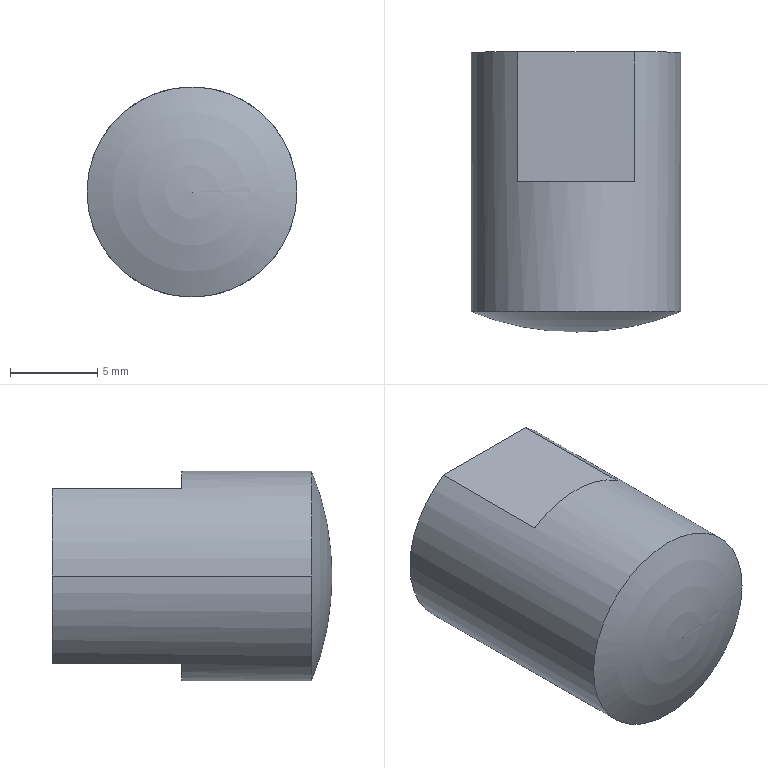Part | NX | 1 solid | 12 faces | box 12 x 16 x 12 mm | volume 1561 mm3 | plane 5 | cylinder 4 | cone 2 | sphere 1 | commonest cylinder face diameters 4.2 x2 12 x2
STEP:
#1=CARTESIAN_POINT('',(6.,-2.832,0.));
#2=VERTEX_POINT('',#1);
#3=CARTESIAN_POINT('',(-6.,-2.832,0.));
#4=VERTEX_POINT('',#3);
#5=CARTESIAN_POINT('',(0.,-2.832,0.));
#6=DIRECTION('',(0.,1.,0.));
#7=DIRECTION('',(1.,0.,0.));
#8=AXIS2_PLACEMENT_3D('',#5,#6,#7);
#9=CIRCLE('',#8,6.);
#10=EDGE_CURVE('',#2,#4,#9,.T.);
#11=ORIENTED_EDGE('',*,*,#10,.F.);
#12=CARTESIAN_POINT('',(0.,-2.832,0.));
#13=DIRECTION('',(0.,1.,0.));
#14=DIRECTION('',(1.,0.,0.));
#15=AXIS2_PLACEMENT_3D('',#12,#13,#14);
#16=CIRCLE('',#15,6.);
#17=EDGE_CURVE('',#4,#2,#16,.T.);
#18=ORIENTED_EDGE('',*,*,#17,.F.);
#19=EDGE_LOOP('',(#11,#18));
#20=FACE_BOUND('',#19,.T.);
#21=CARTESIAN_POINT('',(0.,12.,0.));
#22=DIRECTION('',(0.,1.,0.));
#23=DIRECTION('',(1.,0.,0.));
#24=AXIS2_PLACEMENT_3D('',#21,#22,#23);
#25=SPHERICAL_SURFACE('',#24,16.);
#26=ADVANCED_FACE('',(#20),#25,.T.);
#27=CARTESIAN_POINT('',(-2.1,4.,0.));
#28=VERTEX_POINT('',#27);
#29=CARTESIAN_POINT('',(2.1,4.,0.));
#30=VERTEX_POINT('',#29);
#31=CARTESIAN_POINT('',(0.,4.,0.));
#32=DIRECTION('',(0.,-1.,0.));
#33=DIRECTION('',(1.,0.,0.));
#34=AXIS2_PLACEMENT_3D('',#31,#32,#33);
#35=CIRCLE('',#34,2.1);
#36=EDGE_CURVE('',#28,#30,#35,.T.);
#37=ORIENTED_EDGE('',*,*,#36,.T.);
#38=CARTESIAN_POINT('',(2.1,12.,0.));
#39=VERTEX_POINT('',#38);
#40=CARTESIAN_POINT('',(2.1,2.275,0.));
#41=DIRECTION('',(0.,1.,0.));
#42=VECTOR('',#41,1000.);
#43=LINE('',#40,#42);
#44=EDGE_CURVE('',#30,#39,#43,.T.);
#45=ORIENTED_EDGE('',*,*,#44,.T.);
#46=CARTESIAN_POINT('',(-2.1,12.,0.));
#47=VERTEX_POINT('',#46);
#48=CARTESIAN_POINT('',(0.,12.,0.));
#49=DIRECTION('',(0.,1.,0.));
#50=DIRECTION('',(-1.,0.,0.));
#51=AXIS2_PLACEMENT_3D('',#48,#49,#50);
#52=CIRCLE('',#51,2.1);
#53=EDGE_CURVE('',#39,#47,#52,.T.);
#54=ORIENTED_EDGE('',*,*,#53,.T.);
#55=CARTESIAN_POINT('',(-2.1,2.275,0.));
#56=DIRECTION('',(0.,1.,0.));
#57=VECTOR('',#56,1000.);
#58=LINE('',#55,#57);
#59=EDGE_CURVE('',#28,#47,#58,.T.);
#60=ORIENTED_EDGE('',*,*,#59,.F.);
#61=EDGE_LOOP('',(#37,#45,#54,#60));
#62=FACE_BOUND('',#61,.T.);
#63=CARTESIAN_POINT('',(0.,2.275,0.));
#64=DIRECTION('',(0.,1.,0.));
#65=DIRECTION('',(1.,0.,0.));
#66=AXIS2_PLACEMENT_3D('',#63,#64,#65);
#67=CYLINDRICAL_SURFACE('',#66,2.1);
#68=ADVANCED_FACE('',(#62),#67,.F.);
#69=ORIENTED_EDGE('',*,*,#10,.T.);
#70=CARTESIAN_POINT('',(-6.,12.,0.));
#71=VERTEX_POINT('',#70);
#72=CARTESIAN_POINT('',(-6.,12.8,0.));
#73=DIRECTION('',(0.,-1.,0.));
#74=VECTOR('',#73,1000.);
#75=LINE('',#72,#74);
#76=EDGE_CURVE('',#71,#4,#75,.T.);
#77=ORIENTED_EDGE('',*,*,#76,.F.);
#78=CARTESIAN_POINT('',(-3.317,12.,-5.));
#79=VERTEX_POINT('',#78);
#80=CARTESIAN_POINT('',(0.,12.,0.));
#81=DIRECTION('',(0.,-1.,0.));
#82=DIRECTION('',(-1.,0.,0.));
#83=AXIS2_PLACEMENT_3D('',#80,#81,#82);
#84=CIRCLE('',#83,6.);
#85=EDGE_CURVE('',#71,#79,#84,.T.);
#86=ORIENTED_EDGE('',*,*,#85,.T.);
#87=CARTESIAN_POINT('',(-3.317,4.584,-5.));
#88=VERTEX_POINT('',#87);
#89=CARTESIAN_POINT('',(-3.317,4.584,-5.));
#90=DIRECTION('',(0.,1.,0.));
#91=VECTOR('',#90,1000.);
#92=LINE('',#89,#91);
#93=EDGE_CURVE('',#88,#79,#92,.T.);
#94=ORIENTED_EDGE('',*,*,#93,.F.);
#95=CARTESIAN_POINT('',(3.317,4.584,-5.));
#96=VERTEX_POINT('',#95);
#97=CARTESIAN_POINT('',(0.,4.584,0.));
#98=DIRECTION('',(0.,-1.,0.));
#99=DIRECTION('',(-0.5528,0.,-0.8333));
#100=AXIS2_PLACEMENT_3D('',#97,#98,#99);
#101=CIRCLE('',#100,6.);
#102=EDGE_CURVE('',#88,#96,#101,.T.);
#103=ORIENTED_EDGE('',*,*,#102,.T.);
#104=CARTESIAN_POINT('',(3.317,12.,-5.));
#105=VERTEX_POINT('',#104);
#106=CARTESIAN_POINT('',(3.317,12.,-5.));
#107=DIRECTION('',(0.,-1.,0.));
#108=VECTOR('',#107,1000.);
#109=LINE('',#106,#108);
#110=EDGE_CURVE('',#105,#96,#109,.T.);
#111=ORIENTED_EDGE('',*,*,#110,.F.);
#112=CARTESIAN_POINT('',(6.,12.,0.));
#113=VERTEX_POINT('',#112);
#114=CARTESIAN_POINT('',(0.,12.,0.));
#115=DIRECTION('',(0.,-1.,0.));
#116=DIRECTION('',(0.5528,0.,-0.8333));
#117=AXIS2_PLACEMENT_3D('',#114,#115,#116);
#118=CIRCLE('',#117,6.);
#119=EDGE_CURVE('',#105,#113,#118,.T.);
#120=ORIENTED_EDGE('',*,*,#119,.T.);
#121=CARTESIAN_POINT('',(6.,12.8,0.));
#122=DIRECTION('',(0.,-1.,0.));
#123=VECTOR('',#122,1000.);
#124=LINE('',#121,#123);
#125=EDGE_CURVE('',#113,#2,#124,.T.);
#126=ORIENTED_EDGE('',*,*,#125,.T.);
#127=EDGE_LOOP('',(#69,#77,#86,#94,#103,#111,#120,#126));
#128=FACE_BOUND('',#127,.T.);
#129=CARTESIAN_POINT('',(0.,12.8,0.));
#130=DIRECTION('',(0.,-1.,0.));
#131=DIRECTION('',(1.,0.,0.));
#132=AXIS2_PLACEMENT_3D('',#129,#130,#131);
#133=CYLINDRICAL_SURFACE('',#132,6.);
#134=ADVANCED_FACE('',(#128),#133,.T.);
#135=ORIENTED_EDGE('',*,*,#85,.F.);
#136=CARTESIAN_POINT('',(-3.317,12.,5.));
#137=VERTEX_POINT('',#136);
#138=CARTESIAN_POINT('',(0.,12.,0.));
#139=DIRECTION('',(0.,-1.,0.));
#140=DIRECTION('',(-1.,0.,0.));
#141=AXIS2_PLACEMENT_3D('',#138,#139,#140);
#142=CIRCLE('',#141,6.);
#143=EDGE_CURVE('',#137,#71,#142,.T.);
#144=ORIENTED_EDGE('',*,*,#143,.F.);
#145=CARTESIAN_POINT('',(3.317,12.,5.));
#146=VERTEX_POINT('',#145);
#147=CARTESIAN_POINT('',(-3.317,12.,5.));
#148=DIRECTION('',(1.,0.,0.));
#149=VECTOR('',#148,1000.);
#150=LINE('',#147,#149);
#151=EDGE_CURVE('',#137,#146,#150,.T.);
#152=ORIENTED_EDGE('',*,*,#151,.T.);
#153=CARTESIAN_POINT('',(0.,12.,0.));
#154=DIRECTION('',(0.,-1.,0.));
#155=DIRECTION('',(0.5528,0.,-0.8333));
#156=AXIS2_PLACEMENT_3D('',#153,#154,#155);
#157=CIRCLE('',#156,6.);
#158=EDGE_CURVE('',#113,#146,#157,.T.);
#159=ORIENTED_EDGE('',*,*,#158,.F.);
#160=ORIENTED_EDGE('',*,*,#119,.F.);
#161=CARTESIAN_POINT('',(-3.317,12.,-5.));
#162=DIRECTION('',(1.,0.,0.));
#163=VECTOR('',#162,1000.);
#164=LINE('',#161,#163);
#165=EDGE_CURVE('',#79,#105,#164,.T.);
#166=ORIENTED_EDGE('',*,*,#165,.F.);
#167=EDGE_LOOP('',(#135,#144,#152,#159,#160,#166));
#168=FACE_BOUND('',#167,.T.);
#169=ORIENTED_EDGE('',*,*,#53,.F.);
#170=CARTESIAN_POINT('',(0.,12.,0.));
#171=DIRECTION('',(0.,1.,0.));
#172=DIRECTION('',(-1.,0.,0.));
#173=AXIS2_PLACEMENT_3D('',#170,#171,#172);
#174=CIRCLE('',#173,2.1);
#175=EDGE_CURVE('',#47,#39,#174,.T.);
#176=ORIENTED_EDGE('',*,*,#175,.F.);
#177=EDGE_LOOP('',(#169,#176));
#178=FACE_BOUND('',#177,.T.);
#179=CARTESIAN_POINT('',(0.,12.,0.));
#180=DIRECTION('',(0.,-1.,0.));
#181=DIRECTION('',(0.,0.,-1.));
#182=AXIS2_PLACEMENT_3D('',#179,#180,#181);
#183=PLANE('',#182);
#184=ADVANCED_FACE('',(#168,#178),#183,.F.);
#185=CARTESIAN_POINT('',(0.,2.738,0.));
#186=VERTEX_POINT('',#185);
#187=CARTESIAN_POINT('',(-1.071,3.382,0.));
#188=DIRECTION('',(-0.8572,0.515,0.));
#189=VECTOR('',#188,1000.);
#190=LINE('',#187,#189);
#191=EDGE_CURVE('',#28,#186,#190,.F.);
#192=ORIENTED_EDGE('',*,*,#191,.F.);
#193=CARTESIAN_POINT('',(0.,4.,0.));
#194=DIRECTION('',(0.,-1.,0.));
#195=DIRECTION('',(1.,0.,0.));
#196=AXIS2_PLACEMENT_3D('',#193,#194,#195);
#197=CIRCLE('',#196,2.1);
#198=EDGE_CURVE('',#30,#28,#197,.T.);
#199=ORIENTED_EDGE('',*,*,#198,.F.);
#200=CARTESIAN_POINT('',(1.071,3.382,0.));
#201=DIRECTION('',(0.8572,0.515,0.));
#202=VECTOR('',#201,1000.);
#203=LINE('',#200,#202);
#204=EDGE_CURVE('',#30,#186,#203,.F.);
#205=ORIENTED_EDGE('',*,*,#204,.T.);
#206=EDGE_LOOP('',(#192,#199,#205));
#207=FACE_BOUND('',#206,.T.);
#208=CARTESIAN_POINT('',(0.,3.382,0.));
#209=DIRECTION('',(0.,1.,0.));
#210=DIRECTION('',(1.,0.,0.));
#211=AXIS2_PLACEMENT_3D('',#208,#209,#210);
#212=CONICAL_SURFACE('',#211,1.071,1.03);
#213=ADVANCED_FACE('',(#207),#212,.F.);
#214=ORIENTED_EDGE('',*,*,#93,.T.);
#215=ORIENTED_EDGE('',*,*,#165,.T.);
#216=ORIENTED_EDGE('',*,*,#110,.T.);
#217=CARTESIAN_POINT('',(3.317,4.584,-5.));
#218=DIRECTION('',(-1.,0.,0.));
#219=VECTOR('',#218,1000.);
#220=LINE('',#217,#219);
#221=EDGE_CURVE('',#96,#88,#220,.T.);
#222=ORIENTED_EDGE('',*,*,#221,.T.);
#223=EDGE_LOOP('',(#214,#215,#216,#222));
#224=FACE_BOUND('',#223,.T.);
#225=CARTESIAN_POINT('',(-7.2,4.584,-5.));
#226=DIRECTION('',(0.,0.,1.));
#227=DIRECTION('',(1.,0.,0.));
#228=AXIS2_PLACEMENT_3D('',#225,#226,#227);
#229=PLANE('',#228);
#230=ADVANCED_FACE('',(#224),#229,.F.);
#231=ORIENTED_EDGE('',*,*,#102,.F.);
#232=ORIENTED_EDGE('',*,*,#221,.F.);
#233=EDGE_LOOP('',(#231,#232));
#234=FACE_BOUND('',#233,.T.);
#235=CARTESIAN_POINT('',(-7.2,4.584,-6.));
#236=DIRECTION('',(0.,-1.,0.));
#237=DIRECTION('',(0.,0.,-1.));
#238=AXIS2_PLACEMENT_3D('',#235,#236,#237);
#239=PLANE('',#238);
#240=ADVANCED_FACE('',(#234),#239,.F.);
#241=ORIENTED_EDGE('',*,*,#151,.F.);
#242=CARTESIAN_POINT('',(-3.317,4.584,5.));
#243=VERTEX_POINT('',#242);
#244=CARTESIAN_POINT('',(-3.317,12.,5.));
#245=DIRECTION('',(0.,-1.,0.));
#246=VECTOR('',#245,1000.);
#247=LINE('',#244,#246);
#248=EDGE_CURVE('',#137,#243,#247,.T.);
#249=ORIENTED_EDGE('',*,*,#248,.T.);
#250=CARTESIAN_POINT('',(3.317,4.584,5.));
#251=VERTEX_POINT('',#250);
#252=CARTESIAN_POINT('',(3.317,4.584,5.));
#253=DIRECTION('',(-1.,0.,0.));
#254=VECTOR('',#253,1000.);
#255=LINE('',#252,#254);
#256=EDGE_CURVE('',#251,#243,#255,.T.);
#257=ORIENTED_EDGE('',*,*,#256,.F.);
#258=CARTESIAN_POINT('',(3.317,4.584,5.));
#259=DIRECTION('',(0.,1.,0.));
#260=VECTOR('',#259,1000.);
#261=LINE('',#258,#260);
#262=EDGE_CURVE('',#251,#146,#261,.T.);
#263=ORIENTED_EDGE('',*,*,#262,.T.);
#264=EDGE_LOOP('',(#241,#249,#257,#263));
#265=FACE_BOUND('',#264,.T.);
#266=CARTESIAN_POINT('',(-7.2,12.,5.));
#267=DIRECTION('',(0.,0.,-1.));
#268=DIRECTION('',(0.,-1.,0.));
#269=AXIS2_PLACEMENT_3D('',#266,#267,#268);
#270=PLANE('',#269);
#271=ADVANCED_FACE('',(#265),#270,.F.);
#272=CARTESIAN_POINT('',(0.,4.584,0.));
#273=DIRECTION('',(0.,-1.,0.));
#274=DIRECTION('',(0.5528,0.,0.8333));
#275=AXIS2_PLACEMENT_3D('',#272,#273,#274);
#276=CIRCLE('',#275,6.);
#277=EDGE_CURVE('',#251,#243,#276,.T.);
#278=ORIENTED_EDGE('',*,*,#277,.F.);
#279=ORIENTED_EDGE('',*,*,#256,.T.);
#280=EDGE_LOOP('',(#278,#279));
#281=FACE_BOUND('',#280,.T.);
#282=CARTESIAN_POINT('',(-7.2,4.584,5.));
#283=DIRECTION('',(0.,-1.,0.));
#284=DIRECTION('',(0.,0.,-1.));
#285=AXIS2_PLACEMENT_3D('',#282,#283,#284);
#286=PLANE('',#285);
#287=ADVANCED_FACE('',(#281),#286,.F.);
#288=ORIENTED_EDGE('',*,*,#44,.F.);
#289=ORIENTED_EDGE('',*,*,#198,.T.);
#290=ORIENTED_EDGE('',*,*,#59,.T.);
#291=ORIENTED_EDGE('',*,*,#175,.T.);
#292=EDGE_LOOP('',(#288,#289,#290,#291));
#293=FACE_BOUND('',#292,.T.);
#294=CARTESIAN_POINT('',(0.,2.275,0.));
#295=DIRECTION('',(0.,1.,0.));
#296=DIRECTION('',(1.,0.,0.));
#297=AXIS2_PLACEMENT_3D('',#294,#295,#296);
#298=CYLINDRICAL_SURFACE('',#297,2.1);
#299=ADVANCED_FACE('',(#293),#298,.F.);
#300=ORIENTED_EDGE('',*,*,#125,.F.);
#301=ORIENTED_EDGE('',*,*,#158,.T.);
#302=ORIENTED_EDGE('',*,*,#262,.F.);
#303=ORIENTED_EDGE('',*,*,#277,.T.);
#304=ORIENTED_EDGE('',*,*,#248,.F.);
#305=ORIENTED_EDGE('',*,*,#143,.T.);
#306=ORIENTED_EDGE('',*,*,#76,.T.);
#307=ORIENTED_EDGE('',*,*,#17,.T.);
#308=EDGE_LOOP('',(#300,#301,#302,#303,#304,#305,#306,#307));
#309=FACE_BOUND('',#308,.T.);
#310=CARTESIAN_POINT('',(0.,12.8,0.));
#311=DIRECTION('',(0.,-1.,0.));
#312=DIRECTION('',(1.,0.,0.));
#313=AXIS2_PLACEMENT_3D('',#310,#311,#312);
#314=CYLINDRICAL_SURFACE('',#313,6.);
#315=ADVANCED_FACE('',(#309),#314,.T.);
#316=ORIENTED_EDGE('',*,*,#36,.F.);
#317=ORIENTED_EDGE('',*,*,#191,.T.);
#318=ORIENTED_EDGE('',*,*,#204,.F.);
#319=EDGE_LOOP('',(#316,#317,#318));
#320=FACE_BOUND('',#319,.T.);
#321=CARTESIAN_POINT('',(0.,3.382,0.));
#322=DIRECTION('',(0.,1.,0.));
#323=DIRECTION('',(1.,0.,0.));
#324=AXIS2_PLACEMENT_3D('',#321,#322,#323);
#325=CONICAL_SURFACE('',#324,1.071,1.03);
#326=ADVANCED_FACE('',(#320),#325,.F.);
#327=CLOSED_SHELL('',(#26,#68,#134,#184,#213,#230,#240,#271,#287,#299,#315,#326));
#328=MANIFOLD_SOLID_BREP('',#327);
#329=(LENGTH_UNIT()NAMED_UNIT(*)SI_UNIT(.MILLI.,.METRE.));
#330=UNCERTAINTY_MEASURE_WITH_UNIT(LENGTH_MEASURE(0.00001),#329,'','');
#331=(NAMED_UNIT(*)PLANE_ANGLE_UNIT()SI_UNIT($,.RADIAN.));
#332=(NAMED_UNIT(*)SI_UNIT($,.STERADIAN.)SOLID_ANGLE_UNIT());
#333=(GEOMETRIC_REPRESENTATION_CONTEXT(3)GLOBAL_UNCERTAINTY_ASSIGNED_CONTEXT((#330))GLOBAL_UNIT_ASSIGNED_CONTEXT((#329,#331,#332))REPRESENTATION_CONTEXT('',''));
#334=ADVANCED_BREP_SHAPE_REPRESENTATION('',(#328),#333);